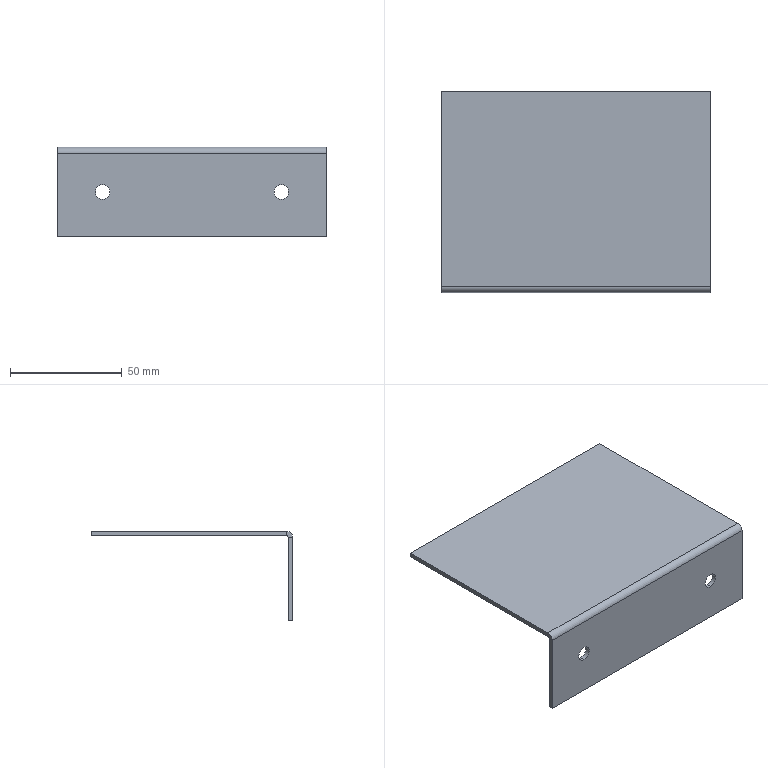Part | STEP file | PN_0016 stop plate | 1 solid | 18 faces | box 120 x 90 x 40 mm | volume 30408 mm3 | plane 12 | cylinder 6 | commonest cylinder face diameters 6.5 x4 1.473 x1 5.473 x1
STEP:
#1=CARTESIAN_POINT('',(0.,0.,0.));
#2=DIRECTION('',(0.,0.,1.));
#3=DIRECTION('',(1.,0.,0.));
#4=AXIS2_PLACEMENT_3D('',#1,#2,#3);
#5=CARTESIAN_POINT('',(40.,0.,-16.75));
#6=VERTEX_POINT('',#5);
#7=CARTESIAN_POINT('',(40.,2.,-16.75));
#8=VERTEX_POINT('',#7);
#9=CARTESIAN_POINT('',(40.,2.,-16.75));
#10=DIRECTION('',(0.,1.,0.));
#11=VECTOR('',#10,1.);
#12=LINE('',#9,#11);
#13=CARTESIAN_POINT('',(40.,2.,-20.));
#14=DIRECTION('',(0.,1.,0.));
#15=DIRECTION('',(0.,0.,1.));
#16=AXIS2_PLACEMENT_3D('',#13,#14,#15);
#17=CYLINDRICAL_SURFACE('',#16,3.25);
#18=CARTESIAN_POINT('',(6.283,0.));
#19=DIRECTION('',(0.,1.));
#20=VECTOR('',#19,1.);
#21=LINE('',#18,#20);
#22=(GEOMETRIC_REPRESENTATION_CONTEXT(2)PARAMETRIC_REPRESENTATION_CONTEXT()REPRESENTATION_CONTEXT('',''));
#23=DEFINITIONAL_REPRESENTATION('',(#21),#22);
#24=PCURVE('',#17,#23);
#25=CARTESIAN_POINT('',(40.,2.,-20.));
#26=DIRECTION('',(0.,1.,0.));
#27=DIRECTION('',(0.,0.,1.));
#28=AXIS2_PLACEMENT_3D('',#25,#26,#27);
#29=CYLINDRICAL_SURFACE('',#28,3.25);
#30=CARTESIAN_POINT('',(0.,0.));
#31=DIRECTION('',(0.,1.));
#32=VECTOR('',#31,1.);
#33=LINE('',#30,#32);
#34=(GEOMETRIC_REPRESENTATION_CONTEXT(2)PARAMETRIC_REPRESENTATION_CONTEXT()REPRESENTATION_CONTEXT('',''));
#35=DEFINITIONAL_REPRESENTATION('',(#33),#34);
#36=PCURVE('',#29,#35);
#37=SURFACE_CURVE('',#12,(#24,#36),.PCURVE_S1.);
#38=EDGE_CURVE('',#6,#8,#37,.T.);
#39=ORIENTED_EDGE('',*,*,#38,.T.);
#40=CARTESIAN_POINT('',(40.,2.,-23.25));
#41=VERTEX_POINT('',#40);
#42=CARTESIAN_POINT('',(40.,2.,-20.));
#43=DIRECTION('',(0.,1.,0.));
#44=DIRECTION('',(0.,0.,1.));
#45=AXIS2_PLACEMENT_3D('',#42,#43,#44);
#46=CIRCLE('',#45,3.25);
#47=CARTESIAN_POINT('',(0.,0.));
#48=DIRECTION('',(1.,0.));
#49=VECTOR('',#48,1.);
#50=LINE('',#47,#49);
#51=(GEOMETRIC_REPRESENTATION_CONTEXT(2)PARAMETRIC_REPRESENTATION_CONTEXT()REPRESENTATION_CONTEXT('',''));
#52=DEFINITIONAL_REPRESENTATION('',(#50),#51);
#53=PCURVE('',#17,#52);
#54=CARTESIAN_POINT('',(60.,2.,0.));
#55=DIRECTION('',(0.,-1.,0.));
#56=DIRECTION('',(0.,0.,-1.));
#57=AXIS2_PLACEMENT_3D('',#54,#55,#56);
#58=PLANE('',#57);
#59=CARTESIAN_POINT('',(16.75,-20.));
#60=CARTESIAN_POINT('',(16.75,-14.371));
#61=CARTESIAN_POINT('',(21.625,-17.185));
#62=CARTESIAN_POINT('',(26.5,-20.));
#63=CARTESIAN_POINT('',(21.625,-22.815));
#64=CARTESIAN_POINT('',(16.75,-25.629));
#65=CARTESIAN_POINT('',(16.75,-20.));
#66=(BOUNDED_CURVE()B_SPLINE_CURVE(2,(#59,#60,#61,#62,#63,#64,#65),.UNSPECIFIED.,.T.,.F.)B_SPLINE_CURVE_WITH_KNOTS((1,2,2,2,2,1),(-2.094,0.,2.094,4.189,6.283,8.378),.UNSPECIFIED.)CURVE()GEOMETRIC_REPRESENTATION_ITEM()RATIONAL_B_SPLINE_CURVE((1.,0.5,1.,0.5,1.,0.5,1.))REPRESENTATION_ITEM(''));
#67=(GEOMETRIC_REPRESENTATION_CONTEXT(2)PARAMETRIC_REPRESENTATION_CONTEXT()REPRESENTATION_CONTEXT('',''));
#68=DEFINITIONAL_REPRESENTATION('',(#66),#67);
#69=PCURVE('',#58,#68);
#70=SURFACE_CURVE('',#46,(#53,#69),.PCURVE_S1.);
#71=EDGE_CURVE('',#41,#8,#70,.T.);
#72=ORIENTED_EDGE('',*,*,#71,.F.);
#73=CARTESIAN_POINT('',(40.,0.,-23.25));
#74=VERTEX_POINT('',#73);
#75=CARTESIAN_POINT('',(40.,2.,-23.25));
#76=DIRECTION('',(0.,1.,0.));
#77=VECTOR('',#76,1.);
#78=LINE('',#75,#77);
#79=CARTESIAN_POINT('',(3.142,0.));
#80=DIRECTION('',(0.,1.));
#81=VECTOR('',#80,1.);
#82=LINE('',#79,#81);
#83=(GEOMETRIC_REPRESENTATION_CONTEXT(2)PARAMETRIC_REPRESENTATION_CONTEXT()REPRESENTATION_CONTEXT('',''));
#84=DEFINITIONAL_REPRESENTATION('',(#82),#83);
#85=PCURVE('',#17,#84);
#86=CARTESIAN_POINT('',(3.142,0.));
#87=DIRECTION('',(0.,1.));
#88=VECTOR('',#87,1.);
#89=LINE('',#86,#88);
#90=(GEOMETRIC_REPRESENTATION_CONTEXT(2)PARAMETRIC_REPRESENTATION_CONTEXT()REPRESENTATION_CONTEXT('',''));
#91=DEFINITIONAL_REPRESENTATION('',(#89),#90);
#92=PCURVE('',#29,#91);
#93=SURFACE_CURVE('',#78,(#85,#92),.PCURVE_S1.);
#94=EDGE_CURVE('',#74,#41,#93,.T.);
#95=ORIENTED_EDGE('',*,*,#94,.F.);
#96=CARTESIAN_POINT('',(40.,0.,-20.));
#97=DIRECTION('',(0.,1.,0.));
#98=DIRECTION('',(0.,0.,1.));
#99=AXIS2_PLACEMENT_3D('',#96,#97,#98);
#100=CIRCLE('',#99,3.25);
#101=CARTESIAN_POINT('',(0.,-2.));
#102=DIRECTION('',(1.,0.));
#103=VECTOR('',#102,1.);
#104=LINE('',#101,#103);
#105=(GEOMETRIC_REPRESENTATION_CONTEXT(2)PARAMETRIC_REPRESENTATION_CONTEXT()REPRESENTATION_CONTEXT('',''));
#106=DEFINITIONAL_REPRESENTATION('',(#104),#105);
#107=PCURVE('',#17,#106);
#108=CARTESIAN_POINT('',(60.,0.,0.));
#109=DIRECTION('',(0.,-1.,0.));
#110=DIRECTION('',(0.,0.,-1.));
#111=AXIS2_PLACEMENT_3D('',#108,#109,#110);
#112=PLANE('',#111);
#113=CARTESIAN_POINT('',(16.75,-20.));
#114=CARTESIAN_POINT('',(16.75,-14.371));
#115=CARTESIAN_POINT('',(21.625,-17.185));
#116=CARTESIAN_POINT('',(26.5,-20.));
#117=CARTESIAN_POINT('',(21.625,-22.815));
#118=CARTESIAN_POINT('',(16.75,-25.629));
#119=CARTESIAN_POINT('',(16.75,-20.));
#120=(BOUNDED_CURVE()B_SPLINE_CURVE(2,(#113,#114,#115,#116,#117,#118,#119),.UNSPECIFIED.,.T.,.F.)B_SPLINE_CURVE_WITH_KNOTS((1,2,2,2,2,1),(-2.094,0.,2.094,4.189,6.283,8.378),.UNSPECIFIED.)CURVE()GEOMETRIC_REPRESENTATION_ITEM()RATIONAL_B_SPLINE_CURVE((1.,0.5,1.,0.5,1.,0.5,1.))REPRESENTATION_ITEM(''));
#121=(GEOMETRIC_REPRESENTATION_CONTEXT(2)PARAMETRIC_REPRESENTATION_CONTEXT()REPRESENTATION_CONTEXT('',''));
#122=DEFINITIONAL_REPRESENTATION('',(#120),#121);
#123=PCURVE('',#112,#122);
#124=SURFACE_CURVE('',#100,(#107,#123),.PCURVE_S1.);
#125=EDGE_CURVE('',#74,#6,#124,.T.);
#126=ORIENTED_EDGE('',*,*,#125,.T.);
#127=EDGE_LOOP('',(#39,#72,#95,#126));
#128=FACE_BOUND('',#127,.F.);
#129=ADVANCED_FACE('',(#128),#17,.F.);
#130=CARTESIAN_POINT('',(-40.,0.,-16.75));
#131=VERTEX_POINT('',#130);
#132=CARTESIAN_POINT('',(-40.,2.,-16.75));
#133=VERTEX_POINT('',#132);
#134=CARTESIAN_POINT('',(-40.,2.,-16.75));
#135=DIRECTION('',(0.,1.,0.));
#136=VECTOR('',#135,1.);
#137=LINE('',#134,#136);
#138=CARTESIAN_POINT('',(-40.,2.,-20.));
#139=DIRECTION('',(0.,1.,0.));
#140=DIRECTION('',(0.,0.,1.));
#141=AXIS2_PLACEMENT_3D('',#138,#139,#140);
#142=CYLINDRICAL_SURFACE('',#141,3.25);
#143=CARTESIAN_POINT('',(6.283,0.));
#144=DIRECTION('',(0.,1.));
#145=VECTOR('',#144,1.);
#146=LINE('',#143,#145);
#147=(GEOMETRIC_REPRESENTATION_CONTEXT(2)PARAMETRIC_REPRESENTATION_CONTEXT()REPRESENTATION_CONTEXT('',''));
#148=DEFINITIONAL_REPRESENTATION('',(#146),#147);
#149=PCURVE('',#142,#148);
#150=CARTESIAN_POINT('',(-40.,2.,-20.));
#151=DIRECTION('',(0.,1.,0.));
#152=DIRECTION('',(0.,0.,1.));
#153=AXIS2_PLACEMENT_3D('',#150,#151,#152);
#154=CYLINDRICAL_SURFACE('',#153,3.25);
#155=CARTESIAN_POINT('',(0.,0.));
#156=DIRECTION('',(0.,1.));
#157=VECTOR('',#156,1.);
#158=LINE('',#155,#157);
#159=(GEOMETRIC_REPRESENTATION_CONTEXT(2)PARAMETRIC_REPRESENTATION_CONTEXT()REPRESENTATION_CONTEXT('',''));
#160=DEFINITIONAL_REPRESENTATION('',(#158),#159);
#161=PCURVE('',#154,#160);
#162=SURFACE_CURVE('',#137,(#149,#161),.PCURVE_S1.);
#163=EDGE_CURVE('',#131,#133,#162,.T.);
#164=ORIENTED_EDGE('',*,*,#163,.T.);
#165=CARTESIAN_POINT('',(-40.,2.,-23.25));
#166=VERTEX_POINT('',#165);
#167=CARTESIAN_POINT('',(-40.,2.,-20.));
#168=DIRECTION('',(0.,1.,0.));
#169=DIRECTION('',(0.,0.,1.));
#170=AXIS2_PLACEMENT_3D('',#167,#168,#169);
#171=CIRCLE('',#170,3.25);
#172=CARTESIAN_POINT('',(0.,0.));
#173=DIRECTION('',(1.,0.));
#174=VECTOR('',#173,1.);
#175=LINE('',#172,#174);
#176=(GEOMETRIC_REPRESENTATION_CONTEXT(2)PARAMETRIC_REPRESENTATION_CONTEXT()REPRESENTATION_CONTEXT('',''));
#177=DEFINITIONAL_REPRESENTATION('',(#175),#176);
#178=PCURVE('',#142,#177);
#179=CARTESIAN_POINT('',(16.75,-100.));
#180=CARTESIAN_POINT('',(16.75,-94.371));
#181=CARTESIAN_POINT('',(21.625,-97.185));
#182=CARTESIAN_POINT('',(26.5,-100.));
#183=CARTESIAN_POINT('',(21.625,-102.815));
#184=CARTESIAN_POINT('',(16.75,-105.629));
#185=CARTESIAN_POINT('',(16.75,-100.));
#186=(BOUNDED_CURVE()B_SPLINE_CURVE(2,(#179,#180,#181,#182,#183,#184,#185),.UNSPECIFIED.,.T.,.F.)B_SPLINE_CURVE_WITH_KNOTS((1,2,2,2,2,1),(-2.094,0.,2.094,4.189,6.283,8.378),.UNSPECIFIED.)CURVE()GEOMETRIC_REPRESENTATION_ITEM()RATIONAL_B_SPLINE_CURVE((1.,0.5,1.,0.5,1.,0.5,1.))REPRESENTATION_ITEM(''));
#187=(GEOMETRIC_REPRESENTATION_CONTEXT(2)PARAMETRIC_REPRESENTATION_CONTEXT()REPRESENTATION_CONTEXT('',''));
#188=DEFINITIONAL_REPRESENTATION('',(#186),#187);
#189=PCURVE('',#58,#188);
#190=SURFACE_CURVE('',#171,(#178,#189),.PCURVE_S1.);
#191=EDGE_CURVE('',#166,#133,#190,.T.);
#192=ORIENTED_EDGE('',*,*,#191,.F.);
#193=CARTESIAN_POINT('',(-40.,0.,-23.25));
#194=VERTEX_POINT('',#193);
#195=CARTESIAN_POINT('',(-40.,2.,-23.25));
#196=DIRECTION('',(0.,1.,0.));
#197=VECTOR('',#196,1.);
#198=LINE('',#195,#197);
#199=CARTESIAN_POINT('',(3.142,0.));
#200=DIRECTION('',(0.,1.));
#201=VECTOR('',#200,1.);
#202=LINE('',#199,#201);
#203=(GEOMETRIC_REPRESENTATION_CONTEXT(2)PARAMETRIC_REPRESENTATION_CONTEXT()REPRESENTATION_CONTEXT('',''));
#204=DEFINITIONAL_REPRESENTATION('',(#202),#203);
#205=PCURVE('',#142,#204);
#206=CARTESIAN_POINT('',(3.142,0.));
#207=DIRECTION('',(0.,1.));
#208=VECTOR('',#207,1.);
#209=LINE('',#206,#208);
#210=(GEOMETRIC_REPRESENTATION_CONTEXT(2)PARAMETRIC_REPRESENTATION_CONTEXT()REPRESENTATION_CONTEXT('',''));
#211=DEFINITIONAL_REPRESENTATION('',(#209),#210);
#212=PCURVE('',#154,#211);
#213=SURFACE_CURVE('',#198,(#205,#212),.PCURVE_S1.);
#214=EDGE_CURVE('',#194,#166,#213,.T.);
#215=ORIENTED_EDGE('',*,*,#214,.F.);
#216=CARTESIAN_POINT('',(-40.,0.,-20.));
#217=DIRECTION('',(0.,1.,0.));
#218=DIRECTION('',(0.,0.,1.));
#219=AXIS2_PLACEMENT_3D('',#216,#217,#218);
#220=CIRCLE('',#219,3.25);
#221=CARTESIAN_POINT('',(0.,-2.));
#222=DIRECTION('',(1.,0.));
#223=VECTOR('',#222,1.);
#224=LINE('',#221,#223);
#225=(GEOMETRIC_REPRESENTATION_CONTEXT(2)PARAMETRIC_REPRESENTATION_CONTEXT()REPRESENTATION_CONTEXT('',''));
#226=DEFINITIONAL_REPRESENTATION('',(#224),#225);
#227=PCURVE('',#142,#226);
#228=CARTESIAN_POINT('',(16.75,-100.));
#229=CARTESIAN_POINT('',(16.75,-94.371));
#230=CARTESIAN_POINT('',(21.625,-97.185));
#231=CARTESIAN_POINT('',(26.5,-100.));
#232=CARTESIAN_POINT('',(21.625,-102.815));
#233=CARTESIAN_POINT('',(16.75,-105.629));
#234=CARTESIAN_POINT('',(16.75,-100.));
#235=(BOUNDED_CURVE()B_SPLINE_CURVE(2,(#228,#229,#230,#231,#232,#233,#234),.UNSPECIFIED.,.T.,.F.)B_SPLINE_CURVE_WITH_KNOTS((1,2,2,2,2,1),(-2.094,0.,2.094,4.189,6.283,8.378),.UNSPECIFIED.)CURVE()GEOMETRIC_REPRESENTATION_ITEM()RATIONAL_B_SPLINE_CURVE((1.,0.5,1.,0.5,1.,0.5,1.))REPRESENTATION_ITEM(''));
#236=(GEOMETRIC_REPRESENTATION_CONTEXT(2)PARAMETRIC_REPRESENTATION_CONTEXT()REPRESENTATION_CONTEXT('',''));
#237=DEFINITIONAL_REPRESENTATION('',(#235),#236);
#238=PCURVE('',#112,#237);
#239=SURFACE_CURVE('',#220,(#227,#238),.PCURVE_S1.);
#240=EDGE_CURVE('',#194,#131,#239,.T.);
#241=ORIENTED_EDGE('',*,*,#240,.T.);
#242=EDGE_LOOP('',(#164,#192,#215,#241));
#243=FACE_BOUND('',#242,.F.);
#244=ADVANCED_FACE('',(#243),#142,.F.);
#245=CARTESIAN_POINT('',(60.,2.737,0.));
#246=VERTEX_POINT('',#245);
#247=CARTESIAN_POINT('',(60.,2.737,-2.));
#248=VERTEX_POINT('',#247);
#249=CARTESIAN_POINT('',(60.,2.737,0.));
#250=DIRECTION('',(0.,0.,-1.));
#251=VECTOR('',#250,1.);
#252=LINE('',#249,#251);
#253=CARTESIAN_POINT('',(60.,2.737,0.));
#254=DIRECTION('',(1.,0.,0.));
#255=DIRECTION('',(0.,0.,-1.));
#256=AXIS2_PLACEMENT_3D('',#253,#254,#255);
#257=PLANE('',#256);
#258=CARTESIAN_POINT('',(0.,0.));
#259=DIRECTION('',(1.,0.));
#260=VECTOR('',#259,1.);
#261=LINE('',#258,#260);
#262=(GEOMETRIC_REPRESENTATION_CONTEXT(2)PARAMETRIC_REPRESENTATION_CONTEXT()REPRESENTATION_CONTEXT('',''));
#263=DEFINITIONAL_REPRESENTATION('',(#261),#262);
#264=PCURVE('',#257,#263);
#265=CARTESIAN_POINT('',(60.,2.,-2.737));
#266=DIRECTION('',(1.,0.,0.));
#267=DIRECTION('',(0.,0.,-1.));
#268=AXIS2_PLACEMENT_3D('',#265,#266,#267);
#269=PLANE('',#268);
#270=CARTESIAN_POINT('',(-2.737,0.7366));
#271=DIRECTION('',(1.,0.));
#272=VECTOR('',#271,1.);
#273=LINE('',#270,#272);
#274=(GEOMETRIC_REPRESENTATION_CONTEXT(2)PARAMETRIC_REPRESENTATION_CONTEXT()REPRESENTATION_CONTEXT('',''));
#275=DEFINITIONAL_REPRESENTATION('',(#273),#274);
#276=PCURVE('',#269,#275);
#277=SURFACE_CURVE('',#252,(#264,#276),.PCURVE_S1.);
#278=EDGE_CURVE('',#246,#248,#277,.T.);
#279=ORIENTED_EDGE('',*,*,#278,.F.);
#280=CARTESIAN_POINT('',(60.,0.,-2.737));
#281=VERTEX_POINT('',#280);
#282=CARTESIAN_POINT('',(60.,2.737,-2.737));
#283=DIRECTION('',(-1.,0.,0.));
#284=DIRECTION('',(0.,0.,-1.));
#285=AXIS2_PLACEMENT_3D('',#282,#283,#284);
#286=CIRCLE('',#285,2.737);
#287=CARTESIAN_POINT('',(5.473,0.));
#288=CARTESIAN_POINT('',(5.473,-4.74));
#289=CARTESIAN_POINT('',(1.368,-2.37));
#290=CARTESIAN_POINT('',(-2.737,0.));
#291=CARTESIAN_POINT('',(1.368,2.37));
#292=CARTESIAN_POINT('',(5.473,4.74));
#293=CARTESIAN_POINT('',(5.473,0.));
#294=(BOUNDED_CURVE()B_SPLINE_CURVE(2,(#287,#288,#289,#290,#291,#292,#293),.UNSPECIFIED.,.T.,.F.)B_SPLINE_CURVE_WITH_KNOTS((1,2,2,2,2,1),(-2.094,0.,2.094,4.189,6.283,8.378),.UNSPECIFIED.)CURVE()GEOMETRIC_REPRESENTATION_ITEM()RATIONAL_B_SPLINE_CURVE((1.,0.5,1.,0.5,1.,0.5,1.))REPRESENTATION_ITEM(''));
#295=(GEOMETRIC_REPRESENTATION_CONTEXT(2)PARAMETRIC_REPRESENTATION_CONTEXT()REPRESENTATION_CONTEXT('',''));
#296=DEFINITIONAL_REPRESENTATION('',(#294),#295);
#297=PCURVE('',#257,#296);
#298=CARTESIAN_POINT('',(60.,2.737,-2.737));
#299=DIRECTION('',(-1.,0.,0.));
#300=DIRECTION('',(0.,0.,1.));
#301=AXIS2_PLACEMENT_3D('',#298,#299,#300);
#302=CYLINDRICAL_SURFACE('',#301,2.737);
#303=CARTESIAN_POINT('',(3.142,0.));
#304=DIRECTION('',(1.,0.));
#305=VECTOR('',#304,1.);
#306=LINE('',#303,#305);
#307=(GEOMETRIC_REPRESENTATION_CONTEXT(2)PARAMETRIC_REPRESENTATION_CONTEXT()REPRESENTATION_CONTEXT('',''));
#308=DEFINITIONAL_REPRESENTATION('',(#306),#307);
#309=PCURVE('',#302,#308);
#310=SURFACE_CURVE('',#286,(#297,#309),.PCURVE_S1.);
#311=EDGE_CURVE('',#281,#246,#310,.T.);
#312=ORIENTED_EDGE('',*,*,#311,.F.);
#313=CARTESIAN_POINT('',(60.,2.,-2.737));
#314=VERTEX_POINT('',#313);
#315=CARTESIAN_POINT('',(60.,2.,-2.737));
#316=DIRECTION('',(0.,-1.,0.));
#317=VECTOR('',#316,1.);
#318=LINE('',#315,#317);
#319=CARTESIAN_POINT('',(2.737,-0.7366));
#320=DIRECTION('',(0.,-1.));
#321=VECTOR('',#320,1.);
#322=LINE('',#319,#321);
#323=(GEOMETRIC_REPRESENTATION_CONTEXT(2)PARAMETRIC_REPRESENTATION_CONTEXT()REPRESENTATION_CONTEXT('',''));
#324=DEFINITIONAL_REPRESENTATION('',(#322),#323);
#325=PCURVE('',#257,#324);
#326=CARTESIAN_POINT('',(60.,2.737,-2.737));
#327=DIRECTION('',(1.,0.,0.));
#328=DIRECTION('',(0.,0.,-1.));
#329=AXIS2_PLACEMENT_3D('',#326,#327,#328);
#330=PLANE('',#329);
#331=CARTESIAN_POINT('',(0.,-0.7366));
#332=DIRECTION('',(0.,-1.));
#333=VECTOR('',#332,1.);
#334=LINE('',#331,#333);
#335=(GEOMETRIC_REPRESENTATION_CONTEXT(2)PARAMETRIC_REPRESENTATION_CONTEXT()REPRESENTATION_CONTEXT('',''));
#336=DEFINITIONAL_REPRESENTATION('',(#334),#335);
#337=PCURVE('',#330,#336);
#338=SURFACE_CURVE('',#318,(#325,#337),.PCURVE_S1.);
#339=EDGE_CURVE('',#314,#281,#338,.T.);
#340=ORIENTED_EDGE('',*,*,#339,.F.);
#341=CARTESIAN_POINT('',(60.,2.737,-2.737));
#342=DIRECTION('',(-1.,0.,0.));
#343=DIRECTION('',(0.,0.,-1.));
#344=AXIS2_PLACEMENT_3D('',#341,#342,#343);
#345=CIRCLE('',#344,0.7366);
#346=CARTESIAN_POINT('',(3.473,0.));
#347=CARTESIAN_POINT('',(3.473,-1.276));
#348=CARTESIAN_POINT('',(2.368,-0.6379));
#349=CARTESIAN_POINT('',(1.263,0.));
#350=CARTESIAN_POINT('',(2.368,0.6379));
#351=CARTESIAN_POINT('',(3.473,1.276));
#352=CARTESIAN_POINT('',(3.473,0.));
#353=(BOUNDED_CURVE()B_SPLINE_CURVE(2,(#346,#347,#348,#349,#350,#351,#352),.UNSPECIFIED.,.T.,.F.)B_SPLINE_CURVE_WITH_KNOTS((1,2,2,2,2,1),(-2.094,0.,2.094,4.189,6.283,8.378),.UNSPECIFIED.)CURVE()GEOMETRIC_REPRESENTATION_ITEM()RATIONAL_B_SPLINE_CURVE((1.,0.5,1.,0.5,1.,0.5,1.))REPRESENTATION_ITEM(''));
#354=(GEOMETRIC_REPRESENTATION_CONTEXT(2)PARAMETRIC_REPRESENTATION_CONTEXT()REPRESENTATION_CONTEXT('',''));
#355=DEFINITIONAL_REPRESENTATION('',(#353),#354);
#356=PCURVE('',#257,#355);
#357=CARTESIAN_POINT('',(60.,2.737,-2.737));
#358=DIRECTION('',(-1.,0.,0.));
#359=DIRECTION('',(0.,0.,1.));
#360=AXIS2_PLACEMENT_3D('',#357,#358,#359);
#361=CYLINDRICAL_SURFACE('',#360,0.7366);
#362=CARTESIAN_POINT('',(3.142,0.));
#363=DIRECTION('',(1.,0.));
#364=VECTOR('',#363,1.);
#365=LINE('',#362,#364);
#366=(GEOMETRIC_REPRESENTATION_CONTEXT(2)PARAMETRIC_REPRESENTATION_CONTEXT()REPRESENTATION_CONTEXT('',''));
#367=DEFINITIONAL_REPRESENTATION('',(#365),#366);
#368=PCURVE('',#361,#367);
#369=SURFACE_CURVE('',#345,(#356,#368),.PCURVE_S1.);
#370=EDGE_CURVE('',#314,#248,#369,.T.);
#371=ORIENTED_EDGE('',*,*,#370,.T.);
#372=EDGE_LOOP('',(#279,#312,#340,#371));
#373=FACE_BOUND('',#372,.T.);
#374=ADVANCED_FACE('',(#373),#257,.T.);
#375=CARTESIAN_POINT('',(60.,90.,0.));
#376=VERTEX_POINT('',#375);
#377=CARTESIAN_POINT('',(60.,0.,0.));
#378=DIRECTION('',(0.,1.,0.));
#379=VECTOR('',#378,1.);
#380=LINE('',#377,#379);
#381=CARTESIAN_POINT('',(-2.737,-2.));
#382=DIRECTION('',(0.,1.));
#383=VECTOR('',#382,1.);
#384=LINE('',#381,#383);
#385=(GEOMETRIC_REPRESENTATION_CONTEXT(2)PARAMETRIC_REPRESENTATION_CONTEXT()REPRESENTATION_CONTEXT('',''));
#386=DEFINITIONAL_REPRESENTATION('',(#384),#385);
#387=PCURVE('',#269,#386);
#388=CARTESIAN_POINT('',(60.,0.,0.));
#389=DIRECTION('',(0.,0.,1.));
#390=DIRECTION('',(1.,0.,0.));
#391=AXIS2_PLACEMENT_3D('',#388,#389,#390);
#392=PLANE('',#391);
#393=CARTESIAN_POINT('',(0.,0.));
#394=DIRECTION('',(0.,1.));
#395=VECTOR('',#394,1.);
#396=LINE('',#393,#395);
#397=(GEOMETRIC_REPRESENTATION_CONTEXT(2)PARAMETRIC_REPRESENTATION_CONTEXT()REPRESENTATION_CONTEXT('',''));
#398=DEFINITIONAL_REPRESENTATION('',(#396),#397);
#399=PCURVE('',#392,#398);
#400=SURFACE_CURVE('',#380,(#387,#399),.PCURVE_S1.);
#401=EDGE_CURVE('',#246,#376,#400,.T.);
#402=ORIENTED_EDGE('',*,*,#401,.F.);
#403=ORIENTED_EDGE('',*,*,#278,.T.);
#404=CARTESIAN_POINT('',(60.,90.,-2.));
#405=VERTEX_POINT('',#404);
#406=CARTESIAN_POINT('',(60.,0.,-2.));
#407=DIRECTION('',(0.,1.,0.));
#408=VECTOR('',#407,1.);
#409=LINE('',#406,#408);
#410=CARTESIAN_POINT('',(-0.7366,-2.));
#411=DIRECTION('',(0.,1.));
#412=VECTOR('',#411,1.);
#413=LINE('',#410,#412);
#414=(GEOMETRIC_REPRESENTATION_CONTEXT(2)PARAMETRIC_REPRESENTATION_CONTEXT()REPRESENTATION_CONTEXT('',''));
#415=DEFINITIONAL_REPRESENTATION('',(#413),#414);
#416=PCURVE('',#269,#415);
#417=CARTESIAN_POINT('',(60.,0.,-2.));
#418=DIRECTION('',(0.,0.,1.));
#419=DIRECTION('',(1.,0.,0.));
#420=AXIS2_PLACEMENT_3D('',#417,#418,#419);
#421=PLANE('',#420);
#422=CARTESIAN_POINT('',(0.,0.));
#423=DIRECTION('',(0.,1.));
#424=VECTOR('',#423,1.);
#425=LINE('',#422,#424);
#426=(GEOMETRIC_REPRESENTATION_CONTEXT(2)PARAMETRIC_REPRESENTATION_CONTEXT()REPRESENTATION_CONTEXT('',''));
#427=DEFINITIONAL_REPRESENTATION('',(#425),#426);
#428=PCURVE('',#421,#427);
#429=SURFACE_CURVE('',#409,(#416,#428),.PCURVE_S1.);
#430=EDGE_CURVE('',#248,#405,#429,.T.);
#431=ORIENTED_EDGE('',*,*,#430,.T.);
#432=CARTESIAN_POINT('',(60.,90.,0.));
#433=DIRECTION('',(0.,0.,-1.));
#434=VECTOR('',#433,1.);
#435=LINE('',#432,#434);
#436=CARTESIAN_POINT('',(-2.737,88.));
#437=DIRECTION('',(1.,0.));
#438=VECTOR('',#437,1.);
#439=LINE('',#436,#438);
#440=(GEOMETRIC_REPRESENTATION_CONTEXT(2)PARAMETRIC_REPRESENTATION_CONTEXT()REPRESENTATION_CONTEXT('',''));
#441=DEFINITIONAL_REPRESENTATION('',(#439),#440);
#442=PCURVE('',#269,#441);
#443=CARTESIAN_POINT('',(60.,90.,0.));
#444=DIRECTION('',(0.,1.,0.));
#445=DIRECTION('',(0.,0.,1.));
#446=AXIS2_PLACEMENT_3D('',#443,#444,#445);
#447=PLANE('',#446);
#448=CARTESIAN_POINT('',(0.,0.));
#449=DIRECTION('',(-1.,0.));
#450=VECTOR('',#449,1.);
#451=LINE('',#448,#450);
#452=(GEOMETRIC_REPRESENTATION_CONTEXT(2)PARAMETRIC_REPRESENTATION_CONTEXT()REPRESENTATION_CONTEXT('',''));
#453=DEFINITIONAL_REPRESENTATION('',(#451),#452);
#454=PCURVE('',#447,#453);
#455=SURFACE_CURVE('',#435,(#442,#454),.PCURVE_S1.);
#456=EDGE_CURVE('',#376,#405,#455,.T.);
#457=ORIENTED_EDGE('',*,*,#456,.F.);
#458=EDGE_LOOP('',(#402,#403,#431,#457));
#459=FACE_BOUND('',#458,.T.);
#460=ADVANCED_FACE('',(#459),#269,.T.);
#461=CARTESIAN_POINT('',(-60.,0.,-2.737));
#462=VERTEX_POINT('',#461);
#463=CARTESIAN_POINT('',(-60.,2.,-2.737));
#464=VERTEX_POINT('',#463);
#465=CARTESIAN_POINT('',(-60.,0.,-2.737));
#466=DIRECTION('',(0.,1.,0.));
#467=VECTOR('',#466,1.);
#468=LINE('',#465,#467);
#469=CARTESIAN_POINT('',(-60.,0.,-2.737));
#470=DIRECTION('',(-1.,0.,0.));
#471=DIRECTION('',(0.,0.,1.));
#472=AXIS2_PLACEMENT_3D('',#469,#470,#471);
#473=PLANE('',#472);
#474=CARTESIAN_POINT('',(0.,0.));
#475=DIRECTION('',(0.,1.));
#476=VECTOR('',#475,1.);
#477=LINE('',#474,#476);
#478=(GEOMETRIC_REPRESENTATION_CONTEXT(2)PARAMETRIC_REPRESENTATION_CONTEXT()REPRESENTATION_CONTEXT('',''));
#479=DEFINITIONAL_REPRESENTATION('',(#477),#478);
#480=PCURVE('',#473,#479);
#481=CARTESIAN_POINT('',(-60.,2.737,-2.));
#482=DIRECTION('',(-1.,0.,0.));
#483=DIRECTION('',(0.,0.,1.));
#484=AXIS2_PLACEMENT_3D('',#481,#482,#483);
#485=PLANE('',#484);
#486=CARTESIAN_POINT('',(-0.7366,-2.737));
#487=DIRECTION('',(0.,1.));
#488=VECTOR('',#487,1.);
#489=LINE('',#486,#488);
#490=(GEOMETRIC_REPRESENTATION_CONTEXT(2)PARAMETRIC_REPRESENTATION_CONTEXT()REPRESENTATION_CONTEXT('',''));
#491=DEFINITIONAL_REPRESENTATION('',(#489),#490);
#492=PCURVE('',#485,#491);
#493=SURFACE_CURVE('',#468,(#480,#492),.PCURVE_S1.);
#494=EDGE_CURVE('',#462,#464,#493,.T.);
#495=ORIENTED_EDGE('',*,*,#494,.F.);
#496=CARTESIAN_POINT('',(-60.,2.737,0.));
#497=VERTEX_POINT('',#496);
#498=CARTESIAN_POINT('',(-60.,2.737,-2.737));
#499=DIRECTION('',(-1.,0.,0.));
#500=DIRECTION('',(0.,0.,-1.));
#501=AXIS2_PLACEMENT_3D('',#498,#499,#500);
#502=CIRCLE('',#501,2.737);
#503=CARTESIAN_POINT('',(0.,2.737));
#504=DIRECTION('',(-1.,0.));
#505=AXIS2_PLACEMENT_2D('',#503,#504);
#506=CIRCLE('',#505,2.737);
#507=(GEOMETRIC_REPRESENTATION_CONTEXT(2)PARAMETRIC_REPRESENTATION_CONTEXT()REPRESENTATION_CONTEXT('',''));
#508=DEFINITIONAL_REPRESENTATION('',(#506),#507);
#509=PCURVE('',#473,#508);
#510=CARTESIAN_POINT('',(3.142,120.));
#511=DIRECTION('',(1.,0.));
#512=VECTOR('',#511,1.);
#513=LINE('',#510,#512);
#514=(GEOMETRIC_REPRESENTATION_CONTEXT(2)PARAMETRIC_REPRESENTATION_CONTEXT()REPRESENTATION_CONTEXT('',''));
#515=DEFINITIONAL_REPRESENTATION('',(#513),#514);
#516=PCURVE('',#302,#515);
#517=SURFACE_CURVE('',#502,(#509,#516),.PCURVE_S1.);
#518=EDGE_CURVE('',#462,#497,#517,.T.);
#519=ORIENTED_EDGE('',*,*,#518,.T.);
#520=CARTESIAN_POINT('',(-60.,2.737,-2.));
#521=VERTEX_POINT('',#520);
#522=CARTESIAN_POINT('',(-60.,2.737,-2.));
#523=DIRECTION('',(0.,0.,1.));
#524=VECTOR('',#523,1.);
#525=LINE('',#522,#524);
#526=CARTESIAN_POINT('',(0.7366,2.737));
#527=DIRECTION('',(1.,0.));
#528=VECTOR('',#527,1.);
#529=LINE('',#526,#528);
#530=(GEOMETRIC_REPRESENTATION_CONTEXT(2)PARAMETRIC_REPRESENTATION_CONTEXT()REPRESENTATION_CONTEXT('',''));
#531=DEFINITIONAL_REPRESENTATION('',(#529),#530);
#532=PCURVE('',#473,#531);
#533=CARTESIAN_POINT('',(-60.,2.737,-2.737));
#534=DIRECTION('',(1.,0.,0.));
#535=DIRECTION('',(0.,0.,-1.));
#536=AXIS2_PLACEMENT_3D('',#533,#534,#535);
#537=PLANE('',#536);
#538=CARTESIAN_POINT('',(-0.7366,0.));
#539=DIRECTION('',(-1.,0.));
#540=VECTOR('',#539,1.);
#541=LINE('',#538,#540);
#542=(GEOMETRIC_REPRESENTATION_CONTEXT(2)PARAMETRIC_REPRESENTATION_CONTEXT()REPRESENTATION_CONTEXT('',''));
#543=DEFINITIONAL_REPRESENTATION('',(#541),#542);
#544=PCURVE('',#537,#543);
#545=SURFACE_CURVE('',#525,(#532,#544),.PCURVE_S1.);
#546=EDGE_CURVE('',#521,#497,#545,.T.);
#547=ORIENTED_EDGE('',*,*,#546,.F.);
#548=CARTESIAN_POINT('',(-60.,2.737,-2.737));
#549=DIRECTION('',(-1.,0.,0.));
#550=DIRECTION('',(0.,0.,-1.));
#551=AXIS2_PLACEMENT_3D('',#548,#549,#550);
#552=CIRCLE('',#551,0.7366);
#553=CARTESIAN_POINT('',(0.,2.737));
#554=DIRECTION('',(-1.,0.));
#555=AXIS2_PLACEMENT_2D('',#553,#554);
#556=CIRCLE('',#555,0.7366);
#557=(GEOMETRIC_REPRESENTATION_CONTEXT(2)PARAMETRIC_REPRESENTATION_CONTEXT()REPRESENTATION_CONTEXT('',''));
#558=DEFINITIONAL_REPRESENTATION('',(#556),#557);
#559=PCURVE('',#473,#558);
#560=CARTESIAN_POINT('',(3.142,120.));
#561=DIRECTION('',(1.,0.));
#562=VECTOR('',#561,1.);
#563=LINE('',#560,#562);
#564=(GEOMETRIC_REPRESENTATION_CONTEXT(2)PARAMETRIC_REPRESENTATION_CONTEXT()REPRESENTATION_CONTEXT('',''));
#565=DEFINITIONAL_REPRESENTATION('',(#563),#564);
#566=PCURVE('',#361,#565);
#567=SURFACE_CURVE('',#552,(#559,#566),.PCURVE_S1.);
#568=EDGE_CURVE('',#464,#521,#567,.T.);
#569=ORIENTED_EDGE('',*,*,#568,.F.);
#570=EDGE_LOOP('',(#495,#519,#547,#569));
#571=FACE_BOUND('',#570,.T.);
#572=ADVANCED_FACE('',(#571),#473,.T.);
#573=CARTESIAN_POINT('',(-60.,0.,-40.));
#574=VERTEX_POINT('',#573);
#575=CARTESIAN_POINT('',(-60.,0.,0.));
#576=DIRECTION('',(0.,0.,1.));
#577=VECTOR('',#576,1.);
#578=LINE('',#575,#577);
#579=CARTESIAN_POINT('',(2.,-2.737));
#580=DIRECTION('',(1.,0.));
#581=VECTOR('',#580,1.);
#582=LINE('',#579,#581);
#583=(GEOMETRIC_REPRESENTATION_CONTEXT(2)PARAMETRIC_REPRESENTATION_CONTEXT()REPRESENTATION_CONTEXT('',''));
#584=DEFINITIONAL_REPRESENTATION('',(#582),#583);
#585=PCURVE('',#485,#584);
#586=CARTESIAN_POINT('',(0.,-120.));
#587=DIRECTION('',(-1.,0.));
#588=VECTOR('',#587,1.);
#589=LINE('',#586,#588);
#590=(GEOMETRIC_REPRESENTATION_CONTEXT(2)PARAMETRIC_REPRESENTATION_CONTEXT()REPRESENTATION_CONTEXT('',''));
#591=DEFINITIONAL_REPRESENTATION('',(#589),#590);
#592=PCURVE('',#112,#591);
#593=SURFACE_CURVE('',#578,(#585,#592),.PCURVE_S1.);
#594=EDGE_CURVE('',#574,#462,#593,.T.);
#595=ORIENTED_EDGE('',*,*,#594,.T.);
#596=ORIENTED_EDGE('',*,*,#494,.T.);
#597=CARTESIAN_POINT('',(-60.,2.,-40.));
#598=VERTEX_POINT('',#597);
#599=CARTESIAN_POINT('',(-60.,2.,0.));
#600=DIRECTION('',(0.,0.,1.));
#601=VECTOR('',#600,1.);
#602=LINE('',#599,#601);
#603=CARTESIAN_POINT('',(2.,-0.7366));
#604=DIRECTION('',(1.,0.));
#605=VECTOR('',#604,1.);
#606=LINE('',#603,#605);
#607=(GEOMETRIC_REPRESENTATION_CONTEXT(2)PARAMETRIC_REPRESENTATION_CONTEXT()REPRESENTATION_CONTEXT('',''));
#608=DEFINITIONAL_REPRESENTATION('',(#606),#607);
#609=PCURVE('',#485,#608);
#610=CARTESIAN_POINT('',(0.,-120.));
#611=DIRECTION('',(-1.,0.));
#612=VECTOR('',#611,1.);
#613=LINE('',#610,#612);
#614=(GEOMETRIC_REPRESENTATION_CONTEXT(2)PARAMETRIC_REPRESENTATION_CONTEXT()REPRESENTATION_CONTEXT('',''));
#615=DEFINITIONAL_REPRESENTATION('',(#613),#614);
#616=PCURVE('',#58,#615);
#617=SURFACE_CURVE('',#602,(#609,#616),.PCURVE_S1.);
#618=EDGE_CURVE('',#598,#464,#617,.T.);
#619=ORIENTED_EDGE('',*,*,#618,.F.);
#620=CARTESIAN_POINT('',(-60.,2.,-40.));
#621=DIRECTION('',(0.,-1.,0.));
#622=VECTOR('',#621,1.);
#623=LINE('',#620,#622);
#624=CARTESIAN_POINT('',(-38.,-0.7366));
#625=DIRECTION('',(0.,-1.));
#626=VECTOR('',#625,1.);
#627=LINE('',#624,#626);
#628=(GEOMETRIC_REPRESENTATION_CONTEXT(2)PARAMETRIC_REPRESENTATION_CONTEXT()REPRESENTATION_CONTEXT('',''));
#629=DEFINITIONAL_REPRESENTATION('',(#627),#628);
#630=PCURVE('',#485,#629);
#631=CARTESIAN_POINT('',(60.,2.,-40.));
#632=DIRECTION('',(0.,0.,-1.));
#633=DIRECTION('',(-1.,0.,0.));
#634=AXIS2_PLACEMENT_3D('',#631,#632,#633);
#635=PLANE('',#634);
#636=CARTESIAN_POINT('',(120.,0.));
#637=DIRECTION('',(0.,-1.));
#638=VECTOR('',#637,1.);
#639=LINE('',#636,#638);
#640=(GEOMETRIC_REPRESENTATION_CONTEXT(2)PARAMETRIC_REPRESENTATION_CONTEXT()REPRESENTATION_CONTEXT('',''));
#641=DEFINITIONAL_REPRESENTATION('',(#639),#640);
#642=PCURVE('',#635,#641);
#643=SURFACE_CURVE('',#623,(#630,#642),.PCURVE_S1.);
#644=EDGE_CURVE('',#598,#574,#643,.T.);
#645=ORIENTED_EDGE('',*,*,#644,.T.);
#646=EDGE_LOOP('',(#595,#596,#619,#645));
#647=FACE_BOUND('',#646,.T.);
#648=ADVANCED_FACE('',(#647),#485,.T.);
#649=CARTESIAN_POINT('',(-60.,90.,-2.));
#650=VERTEX_POINT('',#649);
#651=CARTESIAN_POINT('',(-60.,0.,-2.));
#652=DIRECTION('',(0.,1.,0.));
#653=VECTOR('',#652,1.);
#654=LINE('',#651,#653);
#655=CARTESIAN_POINT('',(-120.,0.));
#656=DIRECTION('',(0.,1.));
#657=VECTOR('',#656,1.);
#658=LINE('',#655,#657);
#659=(GEOMETRIC_REPRESENTATION_CONTEXT(2)PARAMETRIC_REPRESENTATION_CONTEXT()REPRESENTATION_CONTEXT('',''));
#660=DEFINITIONAL_REPRESENTATION('',(#658),#659);
#661=PCURVE('',#421,#660);
#662=CARTESIAN_POINT('',(-0.7366,-2.737));
#663=DIRECTION('',(0.,1.));
#664=VECTOR('',#663,1.);
#665=LINE('',#662,#664);
#666=(GEOMETRIC_REPRESENTATION_CONTEXT(2)PARAMETRIC_REPRESENTATION_CONTEXT()REPRESENTATION_CONTEXT('',''));
#667=DEFINITIONAL_REPRESENTATION('',(#665),#666);
#668=PCURVE('',#537,#667);
#669=SURFACE_CURVE('',#654,(#661,#668),.PCURVE_S1.);
#670=EDGE_CURVE('',#521,#650,#669,.T.);
#671=ORIENTED_EDGE('',*,*,#670,.T.);
#672=CARTESIAN_POINT('',(60.,90.,-2.));
#673=DIRECTION('',(-1.,0.,0.));
#674=VECTOR('',#673,1.);
#675=LINE('',#672,#674);
#676=CARTESIAN_POINT('',(0.,90.));
#677=DIRECTION('',(-1.,0.));
#678=VECTOR('',#677,1.);
#679=LINE('',#676,#678);
#680=(GEOMETRIC_REPRESENTATION_CONTEXT(2)PARAMETRIC_REPRESENTATION_CONTEXT()REPRESENTATION_CONTEXT('',''));
#681=DEFINITIONAL_REPRESENTATION('',(#679),#680);
#682=PCURVE('',#421,#681);
#683=CARTESIAN_POINT('',(-2.,0.));
#684=DIRECTION('',(0.,-1.));
#685=VECTOR('',#684,1.);
#686=LINE('',#683,#685);
#687=(GEOMETRIC_REPRESENTATION_CONTEXT(2)PARAMETRIC_REPRESENTATION_CONTEXT()REPRESENTATION_CONTEXT('',''));
#688=DEFINITIONAL_REPRESENTATION('',(#686),#687);
#689=PCURVE('',#447,#688);
#690=SURFACE_CURVE('',#675,(#682,#689),.PCURVE_S1.);
#691=EDGE_CURVE('',#405,#650,#690,.T.);
#692=ORIENTED_EDGE('',*,*,#691,.F.);
#693=ORIENTED_EDGE('',*,*,#430,.F.);
#694=CARTESIAN_POINT('',(60.,2.737,-2.));
#695=DIRECTION('',(-1.,0.,0.));
#696=VECTOR('',#695,1.);
#697=LINE('',#694,#696);
#698=CARTESIAN_POINT('',(0.,2.737));
#699=DIRECTION('',(-1.,0.));
#700=VECTOR('',#699,1.);
#701=LINE('',#698,#700);
#702=(GEOMETRIC_REPRESENTATION_CONTEXT(2)PARAMETRIC_REPRESENTATION_CONTEXT()REPRESENTATION_CONTEXT('',''));
#703=DEFINITIONAL_REPRESENTATION('',(#701),#702);
#704=PCURVE('',#421,#703);
#705=CARTESIAN_POINT('',(6.283,0.));
#706=DIRECTION('',(0.,1.));
#707=VECTOR('',#706,1.);
#708=LINE('',#705,#707);
#709=(GEOMETRIC_REPRESENTATION_CONTEXT(2)PARAMETRIC_REPRESENTATION_CONTEXT()REPRESENTATION_CONTEXT('',''));
#710=DEFINITIONAL_REPRESENTATION('',(#708),#709);
#711=PCURVE('',#361,#710);
#712=SURFACE_CURVE('',#697,(#704,#711),.PCURVE_S1.);
#713=EDGE_CURVE('',#248,#521,#712,.T.);
#714=ORIENTED_EDGE('',*,*,#713,.T.);
#715=EDGE_LOOP('',(#671,#692,#693,#714));
#716=FACE_BOUND('',#715,.T.);
#717=ADVANCED_FACE('',(#716),#421,.F.);
#718=CARTESIAN_POINT('',(-60.,90.,0.));
#719=VERTEX_POINT('',#718);
#720=CARTESIAN_POINT('',(-60.,90.,0.));
#721=DIRECTION('',(0.,0.,-1.));
#722=VECTOR('',#721,1.);
#723=LINE('',#720,#722);
#724=CARTESIAN_POINT('',(0.,-120.));
#725=DIRECTION('',(-1.,0.));
#726=VECTOR('',#725,1.);
#727=LINE('',#724,#726);
#728=(GEOMETRIC_REPRESENTATION_CONTEXT(2)PARAMETRIC_REPRESENTATION_CONTEXT()REPRESENTATION_CONTEXT('',''));
#729=DEFINITIONAL_REPRESENTATION('',(#727),#728);
#730=PCURVE('',#447,#729);
#731=CARTESIAN_POINT('',(-2.737,87.263));
#732=DIRECTION('',(1.,0.));
#733=VECTOR('',#732,1.);
#734=LINE('',#731,#733);
#735=(GEOMETRIC_REPRESENTATION_CONTEXT(2)PARAMETRIC_REPRESENTATION_CONTEXT()REPRESENTATION_CONTEXT('',''));
#736=DEFINITIONAL_REPRESENTATION('',(#734),#735);
#737=PCURVE('',#537,#736);
#738=SURFACE_CURVE('',#723,(#730,#737),.PCURVE_S1.);
#739=EDGE_CURVE('',#719,#650,#738,.T.);
#740=ORIENTED_EDGE('',*,*,#739,.F.);
#741=CARTESIAN_POINT('',(60.,90.,0.));
#742=DIRECTION('',(-1.,0.,0.));
#743=VECTOR('',#742,1.);
#744=LINE('',#741,#743);
#745=CARTESIAN_POINT('',(0.,0.));
#746=DIRECTION('',(0.,-1.));
#747=VECTOR('',#746,1.);
#748=LINE('',#745,#747);
#749=(GEOMETRIC_REPRESENTATION_CONTEXT(2)PARAMETRIC_REPRESENTATION_CONTEXT()REPRESENTATION_CONTEXT('',''));
#750=DEFINITIONAL_REPRESENTATION('',(#748),#749);
#751=PCURVE('',#447,#750);
#752=CARTESIAN_POINT('',(0.,90.));
#753=DIRECTION('',(-1.,0.));
#754=VECTOR('',#753,1.);
#755=LINE('',#752,#754);
#756=(GEOMETRIC_REPRESENTATION_CONTEXT(2)PARAMETRIC_REPRESENTATION_CONTEXT()REPRESENTATION_CONTEXT('',''));
#757=DEFINITIONAL_REPRESENTATION('',(#755),#756);
#758=PCURVE('',#392,#757);
#759=SURFACE_CURVE('',#744,(#751,#758),.PCURVE_S1.);
#760=EDGE_CURVE('',#376,#719,#759,.T.);
#761=ORIENTED_EDGE('',*,*,#760,.F.);
#762=ORIENTED_EDGE('',*,*,#456,.T.);
#763=ORIENTED_EDGE('',*,*,#691,.T.);
#764=EDGE_LOOP('',(#740,#761,#762,#763));
#765=FACE_BOUND('',#764,.T.);
#766=ADVANCED_FACE('',(#765),#447,.T.);
#767=CARTESIAN_POINT('',(-60.,0.,0.));
#768=DIRECTION('',(0.,1.,0.));
#769=VECTOR('',#768,1.);
#770=LINE('',#767,#769);
#771=CARTESIAN_POINT('',(-120.,0.));
#772=DIRECTION('',(0.,1.));
#773=VECTOR('',#772,1.);
#774=LINE('',#771,#773);
#775=(GEOMETRIC_REPRESENTATION_CONTEXT(2)PARAMETRIC_REPRESENTATION_CONTEXT()REPRESENTATION_CONTEXT('',''));
#776=DEFINITIONAL_REPRESENTATION('',(#774),#775);
#777=PCURVE('',#392,#776);
#778=CARTESIAN_POINT('',(-2.737,-2.737));
#779=DIRECTION('',(0.,1.));
#780=VECTOR('',#779,1.);
#781=LINE('',#778,#780);
#782=(GEOMETRIC_REPRESENTATION_CONTEXT(2)PARAMETRIC_REPRESENTATION_CONTEXT()REPRESENTATION_CONTEXT('',''));
#783=DEFINITIONAL_REPRESENTATION('',(#781),#782);
#784=PCURVE('',#537,#783);
#785=SURFACE_CURVE('',#770,(#777,#784),.PCURVE_S1.);
#786=EDGE_CURVE('',#497,#719,#785,.T.);
#787=ORIENTED_EDGE('',*,*,#786,.F.);
#788=CARTESIAN_POINT('',(60.,2.737,0.));
#789=DIRECTION('',(-1.,0.,0.));
#790=VECTOR('',#789,1.);
#791=LINE('',#788,#790);
#792=CARTESIAN_POINT('',(0.,2.737));
#793=DIRECTION('',(-1.,0.));
#794=VECTOR('',#793,1.);
#795=LINE('',#792,#794);
#796=(GEOMETRIC_REPRESENTATION_CONTEXT(2)PARAMETRIC_REPRESENTATION_CONTEXT()REPRESENTATION_CONTEXT('',''));
#797=DEFINITIONAL_REPRESENTATION('',(#795),#796);
#798=PCURVE('',#392,#797);
#799=CARTESIAN_POINT('',(6.283,0.));
#800=DIRECTION('',(0.,1.));
#801=VECTOR('',#800,1.);
#802=LINE('',#799,#801);
#803=(GEOMETRIC_REPRESENTATION_CONTEXT(2)PARAMETRIC_REPRESENTATION_CONTEXT()REPRESENTATION_CONTEXT('',''));
#804=DEFINITIONAL_REPRESENTATION('',(#802),#803);
#805=PCURVE('',#302,#804);
#806=SURFACE_CURVE('',#791,(#798,#805),.PCURVE_S1.);
#807=EDGE_CURVE('',#246,#497,#806,.T.);
#808=ORIENTED_EDGE('',*,*,#807,.F.);
#809=ORIENTED_EDGE('',*,*,#401,.T.);
#810=ORIENTED_EDGE('',*,*,#760,.T.);
#811=EDGE_LOOP('',(#787,#808,#809,#810));
#812=FACE_BOUND('',#811,.T.);
#813=ADVANCED_FACE('',(#812),#392,.T.);
#814=ORIENTED_EDGE('',*,*,#518,.F.);
#815=CARTESIAN_POINT('',(60.,0.,-2.737));
#816=DIRECTION('',(-1.,0.,0.));
#817=VECTOR('',#816,1.);
#818=LINE('',#815,#817);
#819=CARTESIAN_POINT('',(4.712,0.));
#820=DIRECTION('',(0.,1.));
#821=VECTOR('',#820,1.);
#822=LINE('',#819,#821);
#823=(GEOMETRIC_REPRESENTATION_CONTEXT(2)PARAMETRIC_REPRESENTATION_CONTEXT()REPRESENTATION_CONTEXT('',''));
#824=DEFINITIONAL_REPRESENTATION('',(#822),#823);
#825=PCURVE('',#302,#824);
#826=CARTESIAN_POINT('',(2.737,0.));
#827=DIRECTION('',(0.,-1.));
#828=VECTOR('',#827,1.);
#829=LINE('',#826,#828);
#830=(GEOMETRIC_REPRESENTATION_CONTEXT(2)PARAMETRIC_REPRESENTATION_CONTEXT()REPRESENTATION_CONTEXT('',''));
#831=DEFINITIONAL_REPRESENTATION('',(#829),#830);
#832=PCURVE('',#112,#831);
#833=SURFACE_CURVE('',#818,(#825,#832),.PCURVE_S1.);
#834=EDGE_CURVE('',#281,#462,#833,.T.);
#835=ORIENTED_EDGE('',*,*,#834,.F.);
#836=ORIENTED_EDGE('',*,*,#311,.T.);
#837=ORIENTED_EDGE('',*,*,#807,.T.);
#838=EDGE_LOOP('',(#814,#835,#836,#837));
#839=FACE_BOUND('',#838,.T.);
#840=ADVANCED_FACE('',(#839),#302,.T.);
#841=CARTESIAN_POINT('',(40.,0.,-20.));
#842=DIRECTION('',(0.,1.,0.));
#843=DIRECTION('',(0.,0.,1.));
#844=AXIS2_PLACEMENT_3D('',#841,#842,#843);
#845=CIRCLE('',#844,3.25);
#846=CARTESIAN_POINT('',(16.75,-20.));
#847=CARTESIAN_POINT('',(16.75,-14.371));
#848=CARTESIAN_POINT('',(21.625,-17.185));
#849=CARTESIAN_POINT('',(26.5,-20.));
#850=CARTESIAN_POINT('',(21.625,-22.815));
#851=CARTESIAN_POINT('',(16.75,-25.629));
#852=CARTESIAN_POINT('',(16.75,-20.));
#853=(BOUNDED_CURVE()B_SPLINE_CURVE(2,(#846,#847,#848,#849,#850,#851,#852),.UNSPECIFIED.,.T.,.F.)B_SPLINE_CURVE_WITH_KNOTS((1,2,2,2,2,1),(-2.094,0.,2.094,4.189,6.283,8.378),.UNSPECIFIED.)CURVE()GEOMETRIC_REPRESENTATION_ITEM()RATIONAL_B_SPLINE_CURVE((1.,0.5,1.,0.5,1.,0.5,1.))REPRESENTATION_ITEM(''));
#854=(GEOMETRIC_REPRESENTATION_CONTEXT(2)PARAMETRIC_REPRESENTATION_CONTEXT()REPRESENTATION_CONTEXT('',''));
#855=DEFINITIONAL_REPRESENTATION('',(#853),#854);
#856=PCURVE('',#112,#855);
#857=CARTESIAN_POINT('',(0.,-2.));
#858=DIRECTION('',(1.,0.));
#859=VECTOR('',#858,1.);
#860=LINE('',#857,#859);
#861=(GEOMETRIC_REPRESENTATION_CONTEXT(2)PARAMETRIC_REPRESENTATION_CONTEXT()REPRESENTATION_CONTEXT('',''));
#862=DEFINITIONAL_REPRESENTATION('',(#860),#861);
#863=PCURVE('',#29,#862);
#864=SURFACE_CURVE('',#845,(#856,#863),.PCURVE_S1.);
#865=EDGE_CURVE('',#6,#74,#864,.T.);
#866=ORIENTED_EDGE('',*,*,#865,.T.);
#867=ORIENTED_EDGE('',*,*,#125,.T.);
#868=EDGE_LOOP('',(#866,#867));
#869=FACE_BOUND('',#868,.T.);
#870=CARTESIAN_POINT('',(-40.,0.,-20.));
#871=DIRECTION('',(0.,1.,0.));
#872=DIRECTION('',(0.,0.,1.));
#873=AXIS2_PLACEMENT_3D('',#870,#871,#872);
#874=CIRCLE('',#873,3.25);
#875=CARTESIAN_POINT('',(16.75,-100.));
#876=CARTESIAN_POINT('',(16.75,-94.371));
#877=CARTESIAN_POINT('',(21.625,-97.185));
#878=CARTESIAN_POINT('',(26.5,-100.));
#879=CARTESIAN_POINT('',(21.625,-102.815));
#880=CARTESIAN_POINT('',(16.75,-105.629));
#881=CARTESIAN_POINT('',(16.75,-100.));
#882=(BOUNDED_CURVE()B_SPLINE_CURVE(2,(#875,#876,#877,#878,#879,#880,#881),.UNSPECIFIED.,.T.,.F.)B_SPLINE_CURVE_WITH_KNOTS((1,2,2,2,2,1),(-2.094,0.,2.094,4.189,6.283,8.378),.UNSPECIFIED.)CURVE()GEOMETRIC_REPRESENTATION_ITEM()RATIONAL_B_SPLINE_CURVE((1.,0.5,1.,0.5,1.,0.5,1.))REPRESENTATION_ITEM(''));
#883=(GEOMETRIC_REPRESENTATION_CONTEXT(2)PARAMETRIC_REPRESENTATION_CONTEXT()REPRESENTATION_CONTEXT('',''));
#884=DEFINITIONAL_REPRESENTATION('',(#882),#883);
#885=PCURVE('',#112,#884);
#886=CARTESIAN_POINT('',(0.,-2.));
#887=DIRECTION('',(1.,0.));
#888=VECTOR('',#887,1.);
#889=LINE('',#886,#888);
#890=(GEOMETRIC_REPRESENTATION_CONTEXT(2)PARAMETRIC_REPRESENTATION_CONTEXT()REPRESENTATION_CONTEXT('',''));
#891=DEFINITIONAL_REPRESENTATION('',(#889),#890);
#892=PCURVE('',#154,#891);
#893=SURFACE_CURVE('',#874,(#885,#892),.PCURVE_S1.);
#894=EDGE_CURVE('',#131,#194,#893,.T.);
#895=ORIENTED_EDGE('',*,*,#894,.T.);
#896=ORIENTED_EDGE('',*,*,#240,.T.);
#897=EDGE_LOOP('',(#895,#896));
#898=FACE_BOUND('',#897,.T.);
#899=ORIENTED_EDGE('',*,*,#594,.F.);
#900=CARTESIAN_POINT('',(60.,0.,-40.));
#901=VERTEX_POINT('',#900);
#902=CARTESIAN_POINT('',(60.,0.,-40.));
#903=DIRECTION('',(-1.,0.,0.));
#904=VECTOR('',#903,1.);
#905=LINE('',#902,#904);
#906=CARTESIAN_POINT('',(40.,0.));
#907=DIRECTION('',(0.,-1.));
#908=VECTOR('',#907,1.);
#909=LINE('',#906,#908);
#910=(GEOMETRIC_REPRESENTATION_CONTEXT(2)PARAMETRIC_REPRESENTATION_CONTEXT()REPRESENTATION_CONTEXT('',''));
#911=DEFINITIONAL_REPRESENTATION('',(#909),#910);
#912=PCURVE('',#112,#911);
#913=CARTESIAN_POINT('',(0.,-2.));
#914=DIRECTION('',(1.,0.));
#915=VECTOR('',#914,1.);
#916=LINE('',#913,#915);
#917=(GEOMETRIC_REPRESENTATION_CONTEXT(2)PARAMETRIC_REPRESENTATION_CONTEXT()REPRESENTATION_CONTEXT('',''));
#918=DEFINITIONAL_REPRESENTATION('',(#916),#917);
#919=PCURVE('',#635,#918);
#920=SURFACE_CURVE('',#905,(#912,#919),.PCURVE_S1.);
#921=EDGE_CURVE('',#901,#574,#920,.T.);
#922=ORIENTED_EDGE('',*,*,#921,.F.);
#923=CARTESIAN_POINT('',(60.,0.,0.));
#924=DIRECTION('',(0.,0.,1.));
#925=VECTOR('',#924,1.);
#926=LINE('',#923,#925);
#927=CARTESIAN_POINT('',(0.,0.));
#928=DIRECTION('',(-1.,0.));
#929=VECTOR('',#928,1.);
#930=LINE('',#927,#929);
#931=(GEOMETRIC_REPRESENTATION_CONTEXT(2)PARAMETRIC_REPRESENTATION_CONTEXT()REPRESENTATION_CONTEXT('',''));
#932=DEFINITIONAL_REPRESENTATION('',(#930),#931);
#933=PCURVE('',#112,#932);
#934=CARTESIAN_POINT('',(-2.737,-2.737));
#935=DIRECTION('',(-1.,0.));
#936=VECTOR('',#935,1.);
#937=LINE('',#934,#936);
#938=(GEOMETRIC_REPRESENTATION_CONTEXT(2)PARAMETRIC_REPRESENTATION_CONTEXT()REPRESENTATION_CONTEXT('',''));
#939=DEFINITIONAL_REPRESENTATION('',(#937),#938);
#940=PCURVE('',#330,#939);
#941=SURFACE_CURVE('',#926,(#933,#940),.PCURVE_S1.);
#942=EDGE_CURVE('',#901,#281,#941,.T.);
#943=ORIENTED_EDGE('',*,*,#942,.T.);
#944=ORIENTED_EDGE('',*,*,#834,.T.);
#945=EDGE_LOOP('',(#899,#922,#943,#944));
#946=FACE_BOUND('',#945,.T.);
#947=ADVANCED_FACE('',(#869,#898,#946),#112,.T.);
#948=ORIENTED_EDGE('',*,*,#644,.F.);
#949=CARTESIAN_POINT('',(60.,2.,-40.));
#950=VERTEX_POINT('',#949);
#951=CARTESIAN_POINT('',(60.,2.,-40.));
#952=DIRECTION('',(-1.,0.,0.));
#953=VECTOR('',#952,1.);
#954=LINE('',#951,#953);
#955=CARTESIAN_POINT('',(0.,0.));
#956=DIRECTION('',(1.,0.));
#957=VECTOR('',#956,1.);
#958=LINE('',#955,#957);
#959=(GEOMETRIC_REPRESENTATION_CONTEXT(2)PARAMETRIC_REPRESENTATION_CONTEXT()REPRESENTATION_CONTEXT('',''));
#960=DEFINITIONAL_REPRESENTATION('',(#958),#959);
#961=PCURVE('',#635,#960);
#962=CARTESIAN_POINT('',(40.,0.));
#963=DIRECTION('',(0.,-1.));
#964=VECTOR('',#963,1.);
#965=LINE('',#962,#964);
#966=(GEOMETRIC_REPRESENTATION_CONTEXT(2)PARAMETRIC_REPRESENTATION_CONTEXT()REPRESENTATION_CONTEXT('',''));
#967=DEFINITIONAL_REPRESENTATION('',(#965),#966);
#968=PCURVE('',#58,#967);
#969=SURFACE_CURVE('',#954,(#961,#968),.PCURVE_S1.);
#970=EDGE_CURVE('',#950,#598,#969,.T.);
#971=ORIENTED_EDGE('',*,*,#970,.F.);
#972=CARTESIAN_POINT('',(60.,2.,-40.));
#973=DIRECTION('',(0.,-1.,0.));
#974=VECTOR('',#973,1.);
#975=LINE('',#972,#974);
#976=CARTESIAN_POINT('',(0.,0.));
#977=DIRECTION('',(0.,-1.));
#978=VECTOR('',#977,1.);
#979=LINE('',#976,#978);
#980=(GEOMETRIC_REPRESENTATION_CONTEXT(2)PARAMETRIC_REPRESENTATION_CONTEXT()REPRESENTATION_CONTEXT('',''));
#981=DEFINITIONAL_REPRESENTATION('',(#979),#980);
#982=PCURVE('',#635,#981);
#983=CARTESIAN_POINT('',(37.263,-0.7366));
#984=DIRECTION('',(0.,-1.));
#985=VECTOR('',#984,1.);
#986=LINE('',#983,#985);
#987=(GEOMETRIC_REPRESENTATION_CONTEXT(2)PARAMETRIC_REPRESENTATION_CONTEXT()REPRESENTATION_CONTEXT('',''));
#988=DEFINITIONAL_REPRESENTATION('',(#986),#987);
#989=PCURVE('',#330,#988);
#990=SURFACE_CURVE('',#975,(#982,#989),.PCURVE_S1.);
#991=EDGE_CURVE('',#950,#901,#990,.T.);
#992=ORIENTED_EDGE('',*,*,#991,.T.);
#993=ORIENTED_EDGE('',*,*,#921,.T.);
#994=EDGE_LOOP('',(#948,#971,#992,#993));
#995=FACE_BOUND('',#994,.T.);
#996=ADVANCED_FACE('',(#995),#635,.T.);
#997=CARTESIAN_POINT('',(40.,2.,-20.));
#998=DIRECTION('',(0.,1.,0.));
#999=DIRECTION('',(0.,0.,1.));
#1000=AXIS2_PLACEMENT_3D('',#997,#998,#999);
#1001=CIRCLE('',#1000,3.25);
#1002=CARTESIAN_POINT('',(16.75,-20.));
#1003=CARTESIAN_POINT('',(16.75,-14.371));
#1004=CARTESIAN_POINT('',(21.625,-17.185));
#1005=CARTESIAN_POINT('',(26.5,-20.));
#1006=CARTESIAN_POINT('',(21.625,-22.815));
#1007=CARTESIAN_POINT('',(16.75,-25.629));
#1008=CARTESIAN_POINT('',(16.75,-20.));
#1009=(BOUNDED_CURVE()B_SPLINE_CURVE(2,(#1002,#1003,#1004,#1005,#1006,#1007,#1008),.UNSPECIFIED.,.T.,.F.)B_SPLINE_CURVE_WITH_KNOTS((1,2,2,2,2,1),(-2.094,0.,2.094,4.189,6.283,8.378),.UNSPECIFIED.)CURVE()GEOMETRIC_REPRESENTATION_ITEM()RATIONAL_B_SPLINE_CURVE((1.,0.5,1.,0.5,1.,0.5,1.))REPRESENTATION_ITEM(''));
#1010=(GEOMETRIC_REPRESENTATION_CONTEXT(2)PARAMETRIC_REPRESENTATION_CONTEXT()REPRESENTATION_CONTEXT('',''));
#1011=DEFINITIONAL_REPRESENTATION('',(#1009),#1010);
#1012=PCURVE('',#58,#1011);
#1013=CARTESIAN_POINT('',(0.,0.));
#1014=DIRECTION('',(1.,0.));
#1015=VECTOR('',#1014,1.);
#1016=LINE('',#1013,#1015);
#1017=(GEOMETRIC_REPRESENTATION_CONTEXT(2)PARAMETRIC_REPRESENTATION_CONTEXT()REPRESENTATION_CONTEXT('',''));
#1018=DEFINITIONAL_REPRESENTATION('',(#1016),#1017);
#1019=PCURVE('',#29,#1018);
#1020=SURFACE_CURVE('',#1001,(#1012,#1019),.PCURVE_S1.);
#1021=EDGE_CURVE('',#8,#41,#1020,.T.);
#1022=ORIENTED_EDGE('',*,*,#1021,.F.);
#1023=ORIENTED_EDGE('',*,*,#71,.F.);
#1024=EDGE_LOOP('',(#1022,#1023));
#1025=FACE_BOUND('',#1024,.T.);
#1026=CARTESIAN_POINT('',(-40.,2.,-20.));
#1027=DIRECTION('',(0.,1.,0.));
#1028=DIRECTION('',(0.,0.,1.));
#1029=AXIS2_PLACEMENT_3D('',#1026,#1027,#1028);
#1030=CIRCLE('',#1029,3.25);
#1031=CARTESIAN_POINT('',(16.75,-100.));
#1032=CARTESIAN_POINT('',(16.75,-94.371));
#1033=CARTESIAN_POINT('',(21.625,-97.185));
#1034=CARTESIAN_POINT('',(26.5,-100.));
#1035=CARTESIAN_POINT('',(21.625,-102.815));
#1036=CARTESIAN_POINT('',(16.75,-105.629));
#1037=CARTESIAN_POINT('',(16.75,-100.));
#1038=(BOUNDED_CURVE()B_SPLINE_CURVE(2,(#1031,#1032,#1033,#1034,#1035,#1036,#1037),.UNSPECIFIED.,.T.,.F.)B_SPLINE_CURVE_WITH_KNOTS((1,2,2,2,2,1),(-2.094,0.,2.094,4.189,6.283,8.378),.UNSPECIFIED.)CURVE()GEOMETRIC_REPRESENTATION_ITEM()RATIONAL_B_SPLINE_CURVE((1.,0.5,1.,0.5,1.,0.5,1.))REPRESENTATION_ITEM(''));
#1039=(GEOMETRIC_REPRESENTATION_CONTEXT(2)PARAMETRIC_REPRESENTATION_CONTEXT()REPRESENTATION_CONTEXT('',''));
#1040=DEFINITIONAL_REPRESENTATION('',(#1038),#1039);
#1041=PCURVE('',#58,#1040);
#1042=CARTESIAN_POINT('',(0.,0.));
#1043=DIRECTION('',(1.,0.));
#1044=VECTOR('',#1043,1.);
#1045=LINE('',#1042,#1044);
#1046=(GEOMETRIC_REPRESENTATION_CONTEXT(2)PARAMETRIC_REPRESENTATION_CONTEXT()REPRESENTATION_CONTEXT('',''));
#1047=DEFINITIONAL_REPRESENTATION('',(#1045),#1046);
#1048=PCURVE('',#154,#1047);
#1049=SURFACE_CURVE('',#1030,(#1041,#1048),.PCURVE_S1.);
#1050=EDGE_CURVE('',#133,#166,#1049,.T.);
#1051=ORIENTED_EDGE('',*,*,#1050,.F.);
#1052=ORIENTED_EDGE('',*,*,#191,.F.);
#1053=EDGE_LOOP('',(#1051,#1052));
#1054=FACE_BOUND('',#1053,.T.);
#1055=ORIENTED_EDGE('',*,*,#618,.T.);
#1056=CARTESIAN_POINT('',(60.,2.,-2.737));
#1057=DIRECTION('',(-1.,0.,0.));
#1058=VECTOR('',#1057,1.);
#1059=LINE('',#1056,#1058);
#1060=CARTESIAN_POINT('',(2.737,0.));
#1061=DIRECTION('',(0.,-1.));
#1062=VECTOR('',#1061,1.);
#1063=LINE('',#1060,#1062);
#1064=(GEOMETRIC_REPRESENTATION_CONTEXT(2)PARAMETRIC_REPRESENTATION_CONTEXT()REPRESENTATION_CONTEXT('',''));
#1065=DEFINITIONAL_REPRESENTATION('',(#1063),#1064);
#1066=PCURVE('',#58,#1065);
#1067=CARTESIAN_POINT('',(4.712,0.));
#1068=DIRECTION('',(0.,1.));
#1069=VECTOR('',#1068,1.);
#1070=LINE('',#1067,#1069);
#1071=(GEOMETRIC_REPRESENTATION_CONTEXT(2)PARAMETRIC_REPRESENTATION_CONTEXT()REPRESENTATION_CONTEXT('',''));
#1072=DEFINITIONAL_REPRESENTATION('',(#1070),#1071);
#1073=PCURVE('',#361,#1072);
#1074=SURFACE_CURVE('',#1059,(#1066,#1073),.PCURVE_S1.);
#1075=EDGE_CURVE('',#314,#464,#1074,.T.);
#1076=ORIENTED_EDGE('',*,*,#1075,.F.);
#1077=CARTESIAN_POINT('',(60.,2.,0.));
#1078=DIRECTION('',(0.,0.,1.));
#1079=VECTOR('',#1078,1.);
#1080=LINE('',#1077,#1079);
#1081=CARTESIAN_POINT('',(0.,0.));
#1082=DIRECTION('',(-1.,0.));
#1083=VECTOR('',#1082,1.);
#1084=LINE('',#1081,#1083);
#1085=(GEOMETRIC_REPRESENTATION_CONTEXT(2)PARAMETRIC_REPRESENTATION_CONTEXT()REPRESENTATION_CONTEXT('',''));
#1086=DEFINITIONAL_REPRESENTATION('',(#1084),#1085);
#1087=PCURVE('',#58,#1086);
#1088=CARTESIAN_POINT('',(-2.737,-0.7366));
#1089=DIRECTION('',(-1.,0.));
#1090=VECTOR('',#1089,1.);
#1091=LINE('',#1088,#1090);
#1092=(GEOMETRIC_REPRESENTATION_CONTEXT(2)PARAMETRIC_REPRESENTATION_CONTEXT()REPRESENTATION_CONTEXT('',''));
#1093=DEFINITIONAL_REPRESENTATION('',(#1091),#1092);
#1094=PCURVE('',#330,#1093);
#1095=SURFACE_CURVE('',#1080,(#1087,#1094),.PCURVE_S1.);
#1096=EDGE_CURVE('',#950,#314,#1095,.T.);
#1097=ORIENTED_EDGE('',*,*,#1096,.F.);
#1098=ORIENTED_EDGE('',*,*,#970,.T.);
#1099=EDGE_LOOP('',(#1055,#1076,#1097,#1098));
#1100=FACE_BOUND('',#1099,.T.);
#1101=ADVANCED_FACE('',(#1025,#1054,#1100),#58,.F.);
#1102=ORIENTED_EDGE('',*,*,#1075,.F.);
#1103=ORIENTED_EDGE('',*,*,#370,.T.);
#1104=ORIENTED_EDGE('',*,*,#713,.T.);
#1105=ORIENTED_EDGE('',*,*,#568,.F.);
#1106=EDGE_LOOP('',(#1102,#1103,#1104,#1105));
#1107=FACE_BOUND('',#1106,.F.);
#1108=ADVANCED_FACE('',(#1107),#361,.F.);
#1109=ORIENTED_EDGE('',*,*,#1096,.T.);
#1110=ORIENTED_EDGE('',*,*,#339,.T.);
#1111=ORIENTED_EDGE('',*,*,#942,.F.);
#1112=ORIENTED_EDGE('',*,*,#991,.F.);
#1113=EDGE_LOOP('',(#1109,#1110,#1111,#1112));
#1114=FACE_BOUND('',#1113,.T.);
#1115=ADVANCED_FACE('',(#1114),#330,.T.);
#1116=ORIENTED_EDGE('',*,*,#670,.F.);
#1117=ORIENTED_EDGE('',*,*,#546,.T.);
#1118=ORIENTED_EDGE('',*,*,#786,.T.);
#1119=ORIENTED_EDGE('',*,*,#739,.T.);
#1120=EDGE_LOOP('',(#1116,#1117,#1118,#1119));
#1121=FACE_BOUND('',#1120,.T.);
#1122=ADVANCED_FACE('',(#1121),#537,.F.);
#1123=ORIENTED_EDGE('',*,*,#1050,.F.);
#1124=ORIENTED_EDGE('',*,*,#163,.F.);
#1125=ORIENTED_EDGE('',*,*,#894,.T.);
#1126=ORIENTED_EDGE('',*,*,#214,.T.);
#1127=EDGE_LOOP('',(#1123,#1124,#1125,#1126));
#1128=FACE_BOUND('',#1127,.F.);
#1129=ADVANCED_FACE('',(#1128),#154,.F.);
#1130=ORIENTED_EDGE('',*,*,#1021,.F.);
#1131=ORIENTED_EDGE('',*,*,#38,.F.);
#1132=ORIENTED_EDGE('',*,*,#865,.T.);
#1133=ORIENTED_EDGE('',*,*,#94,.T.);
#1134=EDGE_LOOP('',(#1130,#1131,#1132,#1133));
#1135=FACE_BOUND('',#1134,.F.);
#1136=ADVANCED_FACE('',(#1135),#29,.F.);
#1137=CLOSED_SHELL('',(#129,#244,#374,#460,#572,#648,#717,#766,#813,#840,#947,#996,#1101,#1108,#1115,#1122,#1129,#1136));
#1138=MANIFOLD_SOLID_BREP('',#1137);
#1139=(LENGTH_UNIT()NAMED_UNIT(*)SI_UNIT(.MILLI.,.METRE.));
#1140=UNCERTAINTY_MEASURE_WITH_UNIT(LENGTH_MEASURE(0.0000001),#1139,'','');
#1141=(NAMED_UNIT(*)PLANE_ANGLE_UNIT()SI_UNIT($,.RADIAN.));
#1142=(NAMED_UNIT(*)SI_UNIT($,.STERADIAN.)SOLID_ANGLE_UNIT());
#1143=(GEOMETRIC_REPRESENTATION_CONTEXT(3)GLOBAL_UNCERTAINTY_ASSIGNED_CONTEXT((#1140))GLOBAL_UNIT_ASSIGNED_CONTEXT((#1139,#1141,#1142))REPRESENTATION_CONTEXT('',''));
#1144=ADVANCED_BREP_SHAPE_REPRESENTATION('',(#4,#1138),#1143);